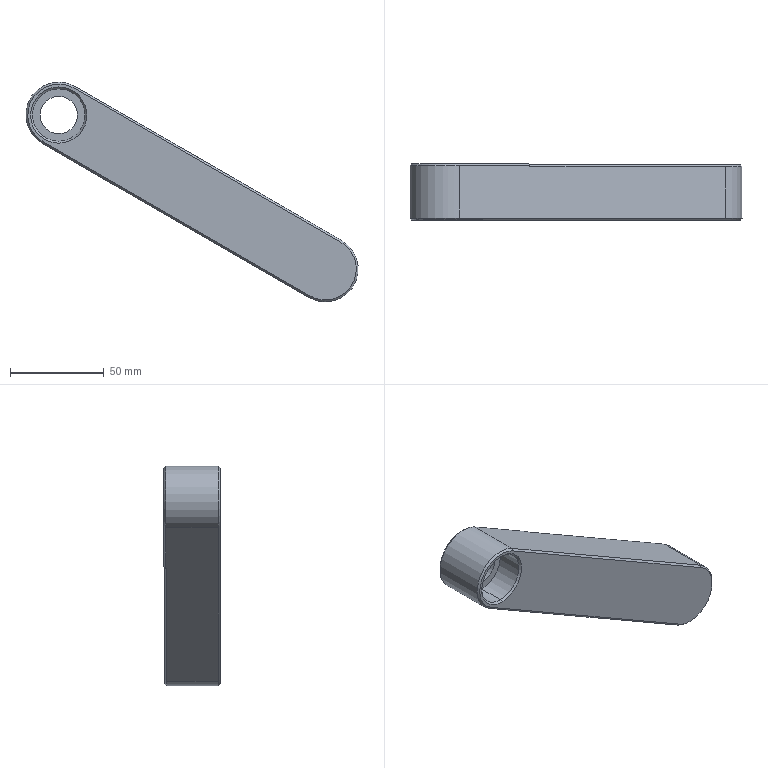Part | Creo | 1 solid | 27 faces | box 177.028 x 30 x 117 mm | volume 184252 mm3 | plane 13 | cone 8 | cylinder 6 | commonest cylinder face diameters 20 x2 28 x2 35 x2
STEP:
#1=CARTESIAN_POINT('',(0.,0.,0.));
#2=DIRECTION('',(0.,0.,1.));
#3=DIRECTION('',(1.,0.,0.));
#4=AXIS2_PLACEMENT_3D('',#1,#2,#3);
#5=CARTESIAN_POINT('',(85.75,-249.,-168.711));
#6=VERTEX_POINT('',#5);
#7=CARTESIAN_POINT('',(-56.278,-249.,-86.711));
#8=VERTEX_POINT('',#7);
#9=CARTESIAN_POINT('',(85.75,-249.,-168.711));
#10=DIRECTION('',(-0.866,0.,0.5));
#11=VECTOR('',#10,164.);
#12=LINE('',#9,#11);
#13=EDGE_CURVE('',#6,#8,#12,.T.);
#14=ORIENTED_EDGE('',*,*,#13,.F.);
#15=CARTESIAN_POINT('',(77.5,-249.,-199.5));
#16=VERTEX_POINT('',#15);
#17=CARTESIAN_POINT('',(77.5,-249.,-183.));
#18=DIRECTION('',(0.,-1.,0.));
#19=DIRECTION('',(0.,0.,-1.));
#20=AXIS2_PLACEMENT_3D('',#17,#18,#19);
#21=CIRCLE('',#20,16.5);
#22=EDGE_CURVE('',#16,#6,#21,.T.);
#23=ORIENTED_EDGE('',*,*,#22,.F.);
#24=CARTESIAN_POINT('',(69.25,-249.,-197.289));
#25=VERTEX_POINT('',#24);
#26=CARTESIAN_POINT('',(77.5,-249.,-183.));
#27=DIRECTION('',(0.,-1.,0.));
#28=DIRECTION('',(-0.5,0.,-0.866));
#29=AXIS2_PLACEMENT_3D('',#26,#27,#28);
#30=CIRCLE('',#29,16.5);
#31=EDGE_CURVE('',#25,#16,#30,.T.);
#32=ORIENTED_EDGE('',*,*,#31,.F.);
#33=CARTESIAN_POINT('',(-72.778,-249.,-115.289));
#34=VERTEX_POINT('',#33);
#35=CARTESIAN_POINT('',(-72.778,-249.,-115.289));
#36=DIRECTION('',(0.866,0.,-0.5));
#37=VECTOR('',#36,164.);
#38=LINE('',#35,#37);
#39=EDGE_CURVE('',#34,#25,#38,.T.);
#40=ORIENTED_EDGE('',*,*,#39,.F.);
#41=CARTESIAN_POINT('',(-64.528,-249.,-101.));
#42=DIRECTION('',(0.,-1.,0.));
#43=DIRECTION('',(0.5,0.,0.866));
#44=AXIS2_PLACEMENT_3D('',#41,#42,#43);
#45=CIRCLE('',#44,16.5);
#46=EDGE_CURVE('',#8,#34,#45,.T.);
#47=ORIENTED_EDGE('',*,*,#46,.F.);
#48=EDGE_LOOP('',(#14,#23,#32,#40,#47));
#49=FACE_OUTER_BOUND('',#48,.F.);
#50=CARTESIAN_POINT('',(-64.528,-249.,-86.));
#51=VERTEX_POINT('',#50);
#52=CARTESIAN_POINT('',(-64.528,-249.,-116.));
#53=VERTEX_POINT('',#52);
#54=CARTESIAN_POINT('',(-64.528,-249.,-101.));
#55=DIRECTION('',(0.,1.,0.));
#56=DIRECTION('',(0.,0.,1.));
#57=AXIS2_PLACEMENT_3D('',#54,#55,#56);
#58=CIRCLE('',#57,15.);
#59=EDGE_CURVE('',#51,#53,#58,.T.);
#60=ORIENTED_EDGE('',*,*,#59,.F.);
#61=CARTESIAN_POINT('',(-64.528,-249.,-101.));
#62=DIRECTION('',(0.,1.,0.));
#63=DIRECTION('',(0.,0.,-1.));
#64=AXIS2_PLACEMENT_3D('',#61,#62,#63);
#65=CIRCLE('',#64,15.);
#66=EDGE_CURVE('',#53,#51,#65,.T.);
#67=ORIENTED_EDGE('',*,*,#66,.F.);
#68=EDGE_LOOP('',(#60,#67));
#69=FACE_BOUND('',#68,.F.);
#70=CARTESIAN_POINT('',(-103.499,-249.,-78.5));
#71=DIRECTION('',(0.,-1.,0.));
#72=DIRECTION('',(0.,0.,-1.));
#73=AXIS2_PLACEMENT_3D('',#70,#71,#72);
#74=PLANE('',#73);
#75=ADVANCED_FACE('',(#49,#69),#74,.T.);
#76=CARTESIAN_POINT('',(-64.528,-248.,-87.));
#77=VERTEX_POINT('',#76);
#78=CARTESIAN_POINT('',(-64.528,-248.,-115.));
#79=VERTEX_POINT('',#78);
#80=CARTESIAN_POINT('',(-64.528,-248.,-101.));
#81=DIRECTION('',(0.,1.,0.));
#82=DIRECTION('',(0.,0.,1.));
#83=AXIS2_PLACEMENT_3D('',#80,#81,#82);
#84=CIRCLE('',#83,14.);
#85=EDGE_CURVE('',#77,#79,#84,.T.);
#86=ORIENTED_EDGE('',*,*,#85,.F.);
#87=CARTESIAN_POINT('',(-64.528,-248.,-87.));
#88=DIRECTION('',(0.,-0.7071,0.7071));
#89=VECTOR('',#88,1.414);
#90=LINE('',#87,#89);
#91=EDGE_CURVE('',#77,#51,#90,.T.);
#92=ORIENTED_EDGE('',*,*,#91,.T.);
#93=ORIENTED_EDGE('',*,*,#59,.T.);
#94=CARTESIAN_POINT('',(-64.528,-248.,-115.));
#95=DIRECTION('',(0.,-0.7071,-0.7071));
#96=VECTOR('',#95,1.414);
#97=LINE('',#94,#96);
#98=EDGE_CURVE('',#79,#53,#97,.T.);
#99=ORIENTED_EDGE('',*,*,#98,.F.);
#100=EDGE_LOOP('',(#86,#92,#93,#99));
#101=FACE_OUTER_BOUND('',#100,.F.);
#102=CARTESIAN_POINT('',(-64.528,-248.5,-101.));
#103=DIRECTION('',(0.,-1.,0.));
#104=DIRECTION('',(0.,0.,1.));
#105=AXIS2_PLACEMENT_3D('',#102,#103,#104);
#106=CONICAL_SURFACE('',#105,14.5,45.);
#107=ADVANCED_FACE('',(#101),#106,.F.);
#108=ORIENTED_EDGE('',*,*,#85,.T.);
#109=CARTESIAN_POINT('',(-64.528,-234.,-115.));
#110=VERTEX_POINT('',#109);
#111=CARTESIAN_POINT('',(-64.528,-248.,-115.));
#112=DIRECTION('',(0.,1.,0.));
#113=VECTOR('',#112,14.);
#114=LINE('',#111,#113);
#115=EDGE_CURVE('',#79,#110,#114,.T.);
#116=ORIENTED_EDGE('',*,*,#115,.T.);
#117=CARTESIAN_POINT('',(-64.528,-234.,-87.));
#118=VERTEX_POINT('',#117);
#119=CARTESIAN_POINT('',(-64.528,-234.,-101.));
#120=DIRECTION('',(0.,-1.,0.));
#121=DIRECTION('',(0.,0.,-1.));
#122=AXIS2_PLACEMENT_3D('',#119,#120,#121);
#123=CIRCLE('',#122,14.);
#124=EDGE_CURVE('',#110,#118,#123,.T.);
#125=ORIENTED_EDGE('',*,*,#124,.T.);
#126=CARTESIAN_POINT('',(-64.528,-248.,-87.));
#127=DIRECTION('',(0.,1.,0.));
#128=VECTOR('',#127,14.);
#129=LINE('',#126,#128);
#130=EDGE_CURVE('',#77,#118,#129,.T.);
#131=ORIENTED_EDGE('',*,*,#130,.F.);
#132=EDGE_LOOP('',(#108,#116,#125,#131));
#133=FACE_OUTER_BOUND('',#132,.F.);
#134=CARTESIAN_POINT('',(-64.528,-249.,-101.));
#135=DIRECTION('',(0.,1.,0.));
#136=DIRECTION('',(0.,0.,1.));
#137=AXIS2_PLACEMENT_3D('',#134,#135,#136);
#138=CYLINDRICAL_SURFACE('',#137,14.);
#139=ADVANCED_FACE('',(#133),#138,.F.);
#140=CARTESIAN_POINT('',(-64.528,-248.,-101.));
#141=DIRECTION('',(0.,1.,0.));
#142=DIRECTION('',(0.,0.,-1.));
#143=AXIS2_PLACEMENT_3D('',#140,#141,#142);
#144=CIRCLE('',#143,14.);
#145=EDGE_CURVE('',#79,#77,#144,.T.);
#146=ORIENTED_EDGE('',*,*,#145,.T.);
#147=ORIENTED_EDGE('',*,*,#130,.T.);
#148=CARTESIAN_POINT('',(-64.528,-234.,-101.));
#149=DIRECTION('',(0.,-1.,0.));
#150=DIRECTION('',(0.,0.,1.));
#151=AXIS2_PLACEMENT_3D('',#148,#149,#150);
#152=CIRCLE('',#151,14.);
#153=EDGE_CURVE('',#118,#110,#152,.T.);
#154=ORIENTED_EDGE('',*,*,#153,.T.);
#155=ORIENTED_EDGE('',*,*,#115,.F.);
#156=EDGE_LOOP('',(#146,#147,#154,#155));
#157=FACE_OUTER_BOUND('',#156,.F.);
#158=CARTESIAN_POINT('',(-64.528,-249.,-101.));
#159=DIRECTION('',(0.,1.,0.));
#160=DIRECTION('',(0.,0.,1.));
#161=AXIS2_PLACEMENT_3D('',#158,#159,#160);
#162=CYLINDRICAL_SURFACE('',#161,14.);
#163=ADVANCED_FACE('',(#157),#162,.F.);
#164=ORIENTED_EDGE('',*,*,#145,.F.);
#165=ORIENTED_EDGE('',*,*,#98,.T.);
#166=ORIENTED_EDGE('',*,*,#66,.T.);
#167=ORIENTED_EDGE('',*,*,#91,.F.);
#168=EDGE_LOOP('',(#164,#165,#166,#167));
#169=FACE_OUTER_BOUND('',#168,.F.);
#170=CARTESIAN_POINT('',(-64.528,-248.5,-101.));
#171=DIRECTION('',(0.,-1.,0.));
#172=DIRECTION('',(0.,0.,1.));
#173=AXIS2_PLACEMENT_3D('',#170,#171,#172);
#174=CONICAL_SURFACE('',#173,14.5,45.);
#175=ADVANCED_FACE('',(#169),#174,.F.);
#176=ORIENTED_EDGE('',*,*,#153,.F.);
#177=ORIENTED_EDGE('',*,*,#124,.F.);
#178=EDGE_LOOP('',(#176,#177));
#179=FACE_OUTER_BOUND('',#178,.F.);
#180=CARTESIAN_POINT('',(-64.528,-234.,-111.));
#181=VERTEX_POINT('',#180);
#182=CARTESIAN_POINT('',(-64.528,-234.,-91.));
#183=VERTEX_POINT('',#182);
#184=CARTESIAN_POINT('',(-64.528,-234.,-101.));
#185=DIRECTION('',(0.,1.,0.));
#186=DIRECTION('',(0.,0.,-1.));
#187=AXIS2_PLACEMENT_3D('',#184,#185,#186);
#188=CIRCLE('',#187,10.);
#189=EDGE_CURVE('',#181,#183,#188,.T.);
#190=ORIENTED_EDGE('',*,*,#189,.F.);
#191=CARTESIAN_POINT('',(-64.528,-234.,-101.));
#192=DIRECTION('',(0.,1.,0.));
#193=DIRECTION('',(0.,0.,1.));
#194=AXIS2_PLACEMENT_3D('',#191,#192,#193);
#195=CIRCLE('',#194,10.);
#196=EDGE_CURVE('',#183,#181,#195,.T.);
#197=ORIENTED_EDGE('',*,*,#196,.F.);
#198=EDGE_LOOP('',(#190,#197));
#199=FACE_BOUND('',#198,.F.);
#200=CARTESIAN_POINT('',(-64.528,-234.,-101.));
#201=DIRECTION('',(0.,-1.,0.));
#202=DIRECTION('',(0.,0.,-1.));
#203=AXIS2_PLACEMENT_3D('',#200,#201,#202);
#204=PLANE('',#203);
#205=ADVANCED_FACE('',(#179,#199),#204,.T.);
#206=CARTESIAN_POINT('',(-64.528,-220.,-91.));
#207=VERTEX_POINT('',#206);
#208=CARTESIAN_POINT('',(-64.528,-220.,-111.));
#209=VERTEX_POINT('',#208);
#210=CARTESIAN_POINT('',(-64.528,-220.,-101.));
#211=DIRECTION('',(0.,-1.,0.));
#212=DIRECTION('',(0.,0.,1.));
#213=AXIS2_PLACEMENT_3D('',#210,#211,#212);
#214=CIRCLE('',#213,10.);
#215=EDGE_CURVE('',#207,#209,#214,.T.);
#216=ORIENTED_EDGE('',*,*,#215,.T.);
#217=CARTESIAN_POINT('',(-64.528,-234.,-111.));
#218=DIRECTION('',(0.,1.,0.));
#219=VECTOR('',#218,14.);
#220=LINE('',#217,#219);
#221=EDGE_CURVE('',#181,#209,#220,.T.);
#222=ORIENTED_EDGE('',*,*,#221,.F.);
#223=ORIENTED_EDGE('',*,*,#189,.T.);
#224=CARTESIAN_POINT('',(-64.528,-234.,-91.));
#225=DIRECTION('',(0.,1.,0.));
#226=VECTOR('',#225,14.);
#227=LINE('',#224,#226);
#228=EDGE_CURVE('',#183,#207,#227,.T.);
#229=ORIENTED_EDGE('',*,*,#228,.T.);
#230=EDGE_LOOP('',(#216,#222,#223,#229));
#231=FACE_OUTER_BOUND('',#230,.F.);
#232=CARTESIAN_POINT('',(-64.528,-249.,-101.));
#233=DIRECTION('',(0.,1.,0.));
#234=DIRECTION('',(0.,0.,1.));
#235=AXIS2_PLACEMENT_3D('',#232,#233,#234);
#236=CYLINDRICAL_SURFACE('',#235,10.);
#237=ADVANCED_FACE('',(#231),#236,.F.);
#238=CARTESIAN_POINT('',(-64.528,-219.,-90.));
#239=VERTEX_POINT('',#238);
#240=CARTESIAN_POINT('',(-64.528,-219.,-112.));
#241=VERTEX_POINT('',#240);
#242=CARTESIAN_POINT('',(-64.528,-219.,-101.));
#243=DIRECTION('',(0.,-1.,0.));
#244=DIRECTION('',(0.,0.,1.));
#245=AXIS2_PLACEMENT_3D('',#242,#243,#244);
#246=CIRCLE('',#245,11.);
#247=EDGE_CURVE('',#239,#241,#246,.T.);
#248=ORIENTED_EDGE('',*,*,#247,.T.);
#249=CARTESIAN_POINT('',(-64.528,-220.,-111.));
#250=DIRECTION('',(0.,0.7071,-0.7071));
#251=VECTOR('',#250,1.414);
#252=LINE('',#249,#251);
#253=EDGE_CURVE('',#209,#241,#252,.T.);
#254=ORIENTED_EDGE('',*,*,#253,.F.);
#255=ORIENTED_EDGE('',*,*,#215,.F.);
#256=CARTESIAN_POINT('',(-64.528,-220.,-91.));
#257=DIRECTION('',(0.,0.7071,0.7071));
#258=VECTOR('',#257,1.414);
#259=LINE('',#256,#258);
#260=EDGE_CURVE('',#207,#239,#259,.T.);
#261=ORIENTED_EDGE('',*,*,#260,.T.);
#262=EDGE_LOOP('',(#248,#254,#255,#261));
#263=FACE_OUTER_BOUND('',#262,.F.);
#264=CARTESIAN_POINT('',(-64.528,-219.5,-101.));
#265=DIRECTION('',(0.,1.,0.));
#266=DIRECTION('',(0.,0.,-1.));
#267=AXIS2_PLACEMENT_3D('',#264,#265,#266);
#268=CONICAL_SURFACE('',#267,10.5,45.);
#269=ADVANCED_FACE('',(#263),#268,.F.);
#270=CARTESIAN_POINT('',(-72.778,-219.,-115.289));
#271=VERTEX_POINT('',#270);
#272=CARTESIAN_POINT('',(-56.278,-219.,-86.711));
#273=VERTEX_POINT('',#272);
#274=CARTESIAN_POINT('',(-64.528,-219.,-101.));
#275=DIRECTION('',(0.,1.,0.));
#276=DIRECTION('',(-0.5,0.,-0.866));
#277=AXIS2_PLACEMENT_3D('',#274,#275,#276);
#278=CIRCLE('',#277,16.5);
#279=EDGE_CURVE('',#271,#273,#278,.T.);
#280=ORIENTED_EDGE('',*,*,#279,.F.);
#281=CARTESIAN_POINT('',(-35.106,-219.,-137.039));
#282=VERTEX_POINT('',#281);
#283=CARTESIAN_POINT('',(-35.106,-219.,-137.039));
#284=DIRECTION('',(-0.866,0.,0.5));
#285=VECTOR('',#284,43.5);
#286=LINE('',#283,#285);
#287=EDGE_CURVE('',#282,#271,#286,.T.);
#288=ORIENTED_EDGE('',*,*,#287,.F.);
#289=CARTESIAN_POINT('',(-18.606,-219.,-108.461));
#290=VERTEX_POINT('',#289);
#291=CARTESIAN_POINT('',(-18.606,-219.,-108.461));
#292=DIRECTION('',(-0.5,0.,-0.866));
#293=VECTOR('',#292,33.);
#294=LINE('',#291,#293);
#295=EDGE_CURVE('',#290,#282,#294,.T.);
#296=ORIENTED_EDGE('',*,*,#295,.F.);
#297=CARTESIAN_POINT('',(-56.278,-219.,-86.711));
#298=DIRECTION('',(0.866,0.,-0.5));
#299=VECTOR('',#298,43.5);
#300=LINE('',#297,#299);
#301=EDGE_CURVE('',#273,#290,#300,.T.);
#302=ORIENTED_EDGE('',*,*,#301,.F.);
#303=EDGE_LOOP('',(#280,#288,#296,#302));
#304=FACE_OUTER_BOUND('',#303,.F.);
#305=ORIENTED_EDGE('',*,*,#247,.F.);
#306=CARTESIAN_POINT('',(-64.528,-219.,-101.));
#307=DIRECTION('',(0.,-1.,0.));
#308=DIRECTION('',(0.,0.,-1.));
#309=AXIS2_PLACEMENT_3D('',#306,#307,#308);
#310=CIRCLE('',#309,11.);
#311=EDGE_CURVE('',#241,#239,#310,.T.);
#312=ORIENTED_EDGE('',*,*,#311,.F.);
#313=EDGE_LOOP('',(#305,#312));
#314=FACE_BOUND('',#313,.F.);
#315=CARTESIAN_POINT('',(-94.839,-219.,-83.5));
#316=DIRECTION('',(0.,-1.,0.));
#317=DIRECTION('',(0.,0.,-1.));
#318=AXIS2_PLACEMENT_3D('',#315,#316,#317);
#319=PLANE('',#318);
#320=ADVANCED_FACE('',(#304,#314),#319,.F.);
#321=ORIENTED_EDGE('',*,*,#311,.T.);
#322=ORIENTED_EDGE('',*,*,#260,.F.);
#323=CARTESIAN_POINT('',(-64.528,-220.,-101.));
#324=DIRECTION('',(0.,-1.,0.));
#325=DIRECTION('',(0.,0.,-1.));
#326=AXIS2_PLACEMENT_3D('',#323,#324,#325);
#327=CIRCLE('',#326,10.);
#328=EDGE_CURVE('',#209,#207,#327,.T.);
#329=ORIENTED_EDGE('',*,*,#328,.F.);
#330=ORIENTED_EDGE('',*,*,#253,.T.);
#331=EDGE_LOOP('',(#321,#322,#329,#330));
#332=FACE_OUTER_BOUND('',#331,.F.);
#333=CARTESIAN_POINT('',(-64.528,-219.5,-101.));
#334=DIRECTION('',(0.,1.,0.));
#335=DIRECTION('',(0.,0.,-1.));
#336=AXIS2_PLACEMENT_3D('',#333,#334,#335);
#337=CONICAL_SURFACE('',#336,10.5,45.);
#338=ADVANCED_FACE('',(#332),#337,.F.);
#339=ORIENTED_EDGE('',*,*,#328,.T.);
#340=ORIENTED_EDGE('',*,*,#228,.F.);
#341=ORIENTED_EDGE('',*,*,#196,.T.);
#342=ORIENTED_EDGE('',*,*,#221,.T.);
#343=EDGE_LOOP('',(#339,#340,#341,#342));
#344=FACE_OUTER_BOUND('',#343,.F.);
#345=CARTESIAN_POINT('',(-64.528,-249.,-101.));
#346=DIRECTION('',(0.,1.,0.));
#347=DIRECTION('',(0.,0.,1.));
#348=AXIS2_PLACEMENT_3D('',#345,#346,#347);
#349=CYLINDRICAL_SURFACE('',#348,10.);
#350=ADVANCED_FACE('',(#344),#349,.F.);
#351=CARTESIAN_POINT('',(-73.278,-220.,-116.155));
#352=VERTEX_POINT('',#351);
#353=CARTESIAN_POINT('',(-72.778,-219.,-115.289));
#354=DIRECTION('',(-0.3536,-0.7071,-0.6124));
#355=VECTOR('',#354,1.414);
#356=LINE('',#353,#355);
#357=EDGE_CURVE('',#271,#352,#356,.T.);
#358=ORIENTED_EDGE('',*,*,#357,.F.);
#359=ORIENTED_EDGE('',*,*,#279,.T.);
#360=CARTESIAN_POINT('',(-55.778,-220.,-85.845));
#361=VERTEX_POINT('',#360);
#362=CARTESIAN_POINT('',(-55.778,-220.,-85.845));
#363=DIRECTION('',(-0.3536,0.7071,-0.6124));
#364=VECTOR('',#363,1.414);
#365=LINE('',#362,#364);
#366=EDGE_CURVE('',#361,#273,#365,.T.);
#367=ORIENTED_EDGE('',*,*,#366,.F.);
#368=CARTESIAN_POINT('',(-64.528,-220.,-83.5));
#369=VERTEX_POINT('',#368);
#370=CARTESIAN_POINT('',(-64.528,-220.,-101.));
#371=DIRECTION('',(0.,1.,0.));
#372=DIRECTION('',(0.,0.,1.));
#373=AXIS2_PLACEMENT_3D('',#370,#371,#372);
#374=CIRCLE('',#373,17.5);
#375=EDGE_CURVE('',#369,#361,#374,.T.);
#376=ORIENTED_EDGE('',*,*,#375,.F.);
#377=CARTESIAN_POINT('',(-64.528,-220.,-101.));
#378=DIRECTION('',(0.,1.,0.));
#379=DIRECTION('',(-0.5,0.,-0.866));
#380=AXIS2_PLACEMENT_3D('',#377,#378,#379);
#381=CIRCLE('',#380,17.5);
#382=EDGE_CURVE('',#352,#369,#381,.T.);
#383=ORIENTED_EDGE('',*,*,#382,.F.);
#384=EDGE_LOOP('',(#358,#359,#367,#376,#383));
#385=FACE_OUTER_BOUND('',#384,.F.);
#386=CARTESIAN_POINT('',(-64.528,-219.5,-101.));
#387=DIRECTION('',(0.,-1.,0.));
#388=DIRECTION('',(0.,0.,1.));
#389=AXIS2_PLACEMENT_3D('',#386,#387,#388);
#390=CONICAL_SURFACE('',#389,17.,45.);
#391=ADVANCED_FACE('',(#385),#390,.T.);
#392=ORIENTED_EDGE('',*,*,#287,.T.);
#393=ORIENTED_EDGE('',*,*,#357,.T.);
#394=CARTESIAN_POINT('',(-35.606,-220.,-137.905));
#395=VERTEX_POINT('',#394);
#396=CARTESIAN_POINT('',(-35.606,-220.,-137.905));
#397=DIRECTION('',(-0.866,0.,0.5));
#398=VECTOR('',#397,43.5);
#399=LINE('',#396,#398);
#400=EDGE_CURVE('',#395,#352,#399,.T.);
#401=ORIENTED_EDGE('',*,*,#400,.F.);
#402=CARTESIAN_POINT('',(-35.606,-220.,-137.905));
#403=DIRECTION('',(0.3536,0.7071,0.6124));
#404=VECTOR('',#403,1.414);
#405=LINE('',#402,#404);
#406=EDGE_CURVE('',#395,#282,#405,.T.);
#407=ORIENTED_EDGE('',*,*,#406,.T.);
#408=EDGE_LOOP('',(#392,#393,#401,#407));
#409=FACE_OUTER_BOUND('',#408,.F.);
#410=CARTESIAN_POINT('',(-103.589,-220.,-98.655));
#411=DIRECTION('',(-0.3536,0.7071,-0.6124));
#412=DIRECTION('',(-0.866,0.,0.5));
#413=AXIS2_PLACEMENT_3D('',#410,#411,#412);
#414=PLANE('',#413);
#415=ADVANCED_FACE('',(#409),#414,.T.);
#416=CARTESIAN_POINT('',(-73.278,-248.,-116.155));
#417=VERTEX_POINT('',#416);
#418=CARTESIAN_POINT('',(68.75,-248.,-198.155));
#419=VERTEX_POINT('',#418);
#420=CARTESIAN_POINT('',(-73.278,-248.,-116.155));
#421=DIRECTION('',(0.866,0.,-0.5));
#422=VECTOR('',#421,164.);
#423=LINE('',#420,#422);
#424=EDGE_CURVE('',#417,#419,#423,.T.);
#425=ORIENTED_EDGE('',*,*,#424,.T.);
#426=CARTESIAN_POINT('',(68.75,-220.5,-198.155));
#427=VERTEX_POINT('',#426);
#428=CARTESIAN_POINT('',(68.75,-248.,-198.155));
#429=DIRECTION('',(0.,1.,0.));
#430=VECTOR('',#429,27.5);
#431=LINE('',#428,#430);
#432=EDGE_CURVE('',#419,#427,#431,.T.);
#433=ORIENTED_EDGE('',*,*,#432,.T.);
#434=CARTESIAN_POINT('',(-35.606,-220.5,-137.905));
#435=VERTEX_POINT('',#434);
#436=CARTESIAN_POINT('',(68.75,-220.5,-198.155));
#437=DIRECTION('',(-0.866,0.,0.5));
#438=VECTOR('',#437,120.5);
#439=LINE('',#436,#438);
#440=EDGE_CURVE('',#427,#435,#439,.T.);
#441=ORIENTED_EDGE('',*,*,#440,.T.);
#442=CARTESIAN_POINT('',(-35.606,-220.,-137.905));
#443=DIRECTION('',(0.,-1.,0.));
#444=VECTOR('',#443,0.5);
#445=LINE('',#442,#444);
#446=EDGE_CURVE('',#395,#435,#445,.T.);
#447=ORIENTED_EDGE('',*,*,#446,.F.);
#448=ORIENTED_EDGE('',*,*,#400,.T.);
#449=CARTESIAN_POINT('',(-73.278,-220.,-116.155));
#450=DIRECTION('',(0.,-1.,0.));
#451=VECTOR('',#450,28.);
#452=LINE('',#449,#451);
#453=EDGE_CURVE('',#352,#417,#452,.T.);
#454=ORIENTED_EDGE('',*,*,#453,.T.);
#455=EDGE_LOOP('',(#425,#433,#441,#447,#448,#454));
#456=FACE_OUTER_BOUND('',#455,.F.);
#457=CARTESIAN_POINT('',(-112.249,-219.,-93.655));
#458=DIRECTION('',(-0.5,0.,-0.866));
#459=DIRECTION('',(-0.866,0.,0.5));
#460=AXIS2_PLACEMENT_3D('',#457,#458,#459);
#461=PLANE('',#460);
#462=ADVANCED_FACE('',(#456),#461,.T.);
#463=ORIENTED_EDGE('',*,*,#39,.T.);
#464=CARTESIAN_POINT('',(69.25,-249.,-197.289));
#465=DIRECTION('',(-0.3536,0.7071,-0.6124));
#466=VECTOR('',#465,1.414);
#467=LINE('',#464,#466);
#468=EDGE_CURVE('',#25,#419,#467,.T.);
#469=ORIENTED_EDGE('',*,*,#468,.T.);
#470=ORIENTED_EDGE('',*,*,#424,.F.);
#471=CARTESIAN_POINT('',(-73.278,-248.,-116.155));
#472=DIRECTION('',(0.3536,-0.7071,0.6124));
#473=VECTOR('',#472,1.414);
#474=LINE('',#471,#473);
#475=EDGE_CURVE('',#417,#34,#474,.T.);
#476=ORIENTED_EDGE('',*,*,#475,.T.);
#477=EDGE_LOOP('',(#463,#469,#470,#476));
#478=FACE_OUTER_BOUND('',#477,.F.);
#479=CARTESIAN_POINT('',(-112.249,-248.,-93.655));
#480=DIRECTION('',(0.3536,0.7071,0.6124));
#481=DIRECTION('',(-0.866,0.,0.5));
#482=AXIS2_PLACEMENT_3D('',#479,#480,#481);
#483=PLANE('',#482);
#484=ADVANCED_FACE('',(#478),#483,.F.);
#485=CARTESIAN_POINT('',(86.25,-248.,-167.845));
#486=VERTEX_POINT('',#485);
#487=CARTESIAN_POINT('',(86.25,-248.,-167.845));
#488=DIRECTION('',(-0.3536,-0.7071,-0.6124));
#489=VECTOR('',#488,1.414);
#490=LINE('',#487,#489);
#491=EDGE_CURVE('',#486,#6,#490,.T.);
#492=ORIENTED_EDGE('',*,*,#491,.F.);
#493=CARTESIAN_POINT('',(77.5,-248.,-200.5));
#494=VERTEX_POINT('',#493);
#495=CARTESIAN_POINT('',(77.5,-248.,-183.));
#496=DIRECTION('',(0.,-1.,0.));
#497=DIRECTION('',(0.,0.,-1.));
#498=AXIS2_PLACEMENT_3D('',#495,#496,#497);
#499=CIRCLE('',#498,17.5);
#500=EDGE_CURVE('',#494,#486,#499,.T.);
#501=ORIENTED_EDGE('',*,*,#500,.F.);
#502=CARTESIAN_POINT('',(77.5,-248.,-183.));
#503=DIRECTION('',(0.,-1.,0.));
#504=DIRECTION('',(-0.5,0.,-0.866));
#505=AXIS2_PLACEMENT_3D('',#502,#503,#504);
#506=CIRCLE('',#505,17.5);
#507=EDGE_CURVE('',#419,#494,#506,.T.);
#508=ORIENTED_EDGE('',*,*,#507,.F.);
#509=ORIENTED_EDGE('',*,*,#468,.F.);
#510=ORIENTED_EDGE('',*,*,#31,.T.);
#511=ORIENTED_EDGE('',*,*,#22,.T.);
#512=EDGE_LOOP('',(#492,#501,#508,#509,#510,#511));
#513=FACE_OUTER_BOUND('',#512,.F.);
#514=CARTESIAN_POINT('',(77.5,-248.5,-183.));
#515=DIRECTION('',(0.,1.,0.));
#516=DIRECTION('',(0.,0.,-1.));
#517=AXIS2_PLACEMENT_3D('',#514,#515,#516);
#518=CONICAL_SURFACE('',#517,17.,45.);
#519=ADVANCED_FACE('',(#513),#518,.T.);
#520=CARTESIAN_POINT('',(-55.778,-248.,-85.845));
#521=VERTEX_POINT('',#520);
#522=CARTESIAN_POINT('',(86.25,-248.,-167.845));
#523=DIRECTION('',(-0.866,0.,0.5));
#524=VECTOR('',#523,164.);
#525=LINE('',#522,#524);
#526=EDGE_CURVE('',#486,#521,#525,.T.);
#527=ORIENTED_EDGE('',*,*,#526,.F.);
#528=ORIENTED_EDGE('',*,*,#491,.T.);
#529=ORIENTED_EDGE('',*,*,#13,.T.);
#530=CARTESIAN_POINT('',(-56.278,-249.,-86.711));
#531=DIRECTION('',(0.3536,0.7071,0.6124));
#532=VECTOR('',#531,1.414);
#533=LINE('',#530,#532);
#534=EDGE_CURVE('',#8,#521,#533,.T.);
#535=ORIENTED_EDGE('',*,*,#534,.T.);
#536=EDGE_LOOP('',(#527,#528,#529,#535));
#537=FACE_OUTER_BOUND('',#536,.F.);
#538=CARTESIAN_POINT('',(-94.749,-248.,-63.345));
#539=DIRECTION('',(0.3536,-0.7071,0.6124));
#540=DIRECTION('',(-0.866,0.,0.5));
#541=AXIS2_PLACEMENT_3D('',#538,#539,#540);
#542=PLANE('',#541);
#543=ADVANCED_FACE('',(#537),#542,.T.);
#544=CARTESIAN_POINT('',(86.25,-220.5,-167.845));
#545=VERTEX_POINT('',#544);
#546=CARTESIAN_POINT('',(86.25,-220.5,-167.845));
#547=DIRECTION('',(0.,-1.,0.));
#548=VECTOR('',#547,27.5);
#549=LINE('',#546,#548);
#550=EDGE_CURVE('',#545,#486,#549,.T.);
#551=ORIENTED_EDGE('',*,*,#550,.T.);
#552=ORIENTED_EDGE('',*,*,#526,.T.);
#553=CARTESIAN_POINT('',(-55.778,-248.,-85.845));
#554=DIRECTION('',(0.,1.,0.));
#555=VECTOR('',#554,28.);
#556=LINE('',#553,#555);
#557=EDGE_CURVE('',#521,#361,#556,.T.);
#558=ORIENTED_EDGE('',*,*,#557,.T.);
#559=CARTESIAN_POINT('',(-18.106,-220.,-107.595));
#560=VERTEX_POINT('',#559);
#561=CARTESIAN_POINT('',(-55.778,-220.,-85.845));
#562=DIRECTION('',(0.866,0.,-0.5));
#563=VECTOR('',#562,43.5);
#564=LINE('',#561,#563);
#565=EDGE_CURVE('',#361,#560,#564,.T.);
#566=ORIENTED_EDGE('',*,*,#565,.T.);
#567=CARTESIAN_POINT('',(-18.106,-220.5,-107.595));
#568=VERTEX_POINT('',#567);
#569=CARTESIAN_POINT('',(-18.106,-220.5,-107.595));
#570=DIRECTION('',(0.,1.,0.));
#571=VECTOR('',#570,0.5);
#572=LINE('',#569,#571);
#573=EDGE_CURVE('',#568,#560,#572,.T.);
#574=ORIENTED_EDGE('',*,*,#573,.F.);
#575=CARTESIAN_POINT('',(-18.106,-220.5,-107.595));
#576=DIRECTION('',(0.866,0.,-0.5));
#577=VECTOR('',#576,120.5);
#578=LINE('',#575,#577);
#579=EDGE_CURVE('',#568,#545,#578,.T.);
#580=ORIENTED_EDGE('',*,*,#579,.T.);
#581=EDGE_LOOP('',(#551,#552,#558,#566,#574,#580));
#582=FACE_OUTER_BOUND('',#581,.F.);
#583=CARTESIAN_POINT('',(-94.749,-219.,-63.345));
#584=DIRECTION('',(-0.5,0.,-0.866));
#585=DIRECTION('',(-0.866,0.,0.5));
#586=AXIS2_PLACEMENT_3D('',#583,#584,#585);
#587=PLANE('',#586);
#588=ADVANCED_FACE('',(#582),#587,.F.);
#589=ORIENTED_EDGE('',*,*,#432,.F.);
#590=ORIENTED_EDGE('',*,*,#507,.T.);
#591=ORIENTED_EDGE('',*,*,#500,.T.);
#592=ORIENTED_EDGE('',*,*,#550,.F.);
#593=CARTESIAN_POINT('',(77.5,-220.5,-200.5));
#594=VERTEX_POINT('',#593);
#595=CARTESIAN_POINT('',(77.5,-220.5,-183.));
#596=DIRECTION('',(0.,1.,0.));
#597=DIRECTION('',(0.5,0.,0.866));
#598=AXIS2_PLACEMENT_3D('',#595,#596,#597);
#599=CIRCLE('',#598,17.5);
#600=EDGE_CURVE('',#545,#594,#599,.T.);
#601=ORIENTED_EDGE('',*,*,#600,.T.);
#602=CARTESIAN_POINT('',(77.5,-220.5,-183.));
#603=DIRECTION('',(0.,1.,0.));
#604=DIRECTION('',(0.,0.,-1.));
#605=AXIS2_PLACEMENT_3D('',#602,#603,#604);
#606=CIRCLE('',#605,17.5);
#607=EDGE_CURVE('',#594,#427,#606,.T.);
#608=ORIENTED_EDGE('',*,*,#607,.T.);
#609=EDGE_LOOP('',(#589,#590,#591,#592,#601,#608));
#610=FACE_OUTER_BOUND('',#609,.F.);
#611=CARTESIAN_POINT('',(77.5,-249.,-183.));
#612=DIRECTION('',(0.,1.,0.));
#613=DIRECTION('',(0.,0.,1.));
#614=AXIS2_PLACEMENT_3D('',#611,#612,#613);
#615=CYLINDRICAL_SURFACE('',#614,17.5);
#616=ADVANCED_FACE('',(#610),#615,.T.);
#617=CARTESIAN_POINT('',(69.25,-219.5,-197.289));
#618=VERTEX_POINT('',#617);
#619=CARTESIAN_POINT('',(68.75,-220.5,-198.155));
#620=DIRECTION('',(0.3536,0.7071,0.6124));
#621=VECTOR('',#620,1.414);
#622=LINE('',#619,#621);
#623=EDGE_CURVE('',#427,#618,#622,.T.);
#624=ORIENTED_EDGE('',*,*,#623,.F.);
#625=ORIENTED_EDGE('',*,*,#607,.F.);
#626=ORIENTED_EDGE('',*,*,#600,.F.);
#627=CARTESIAN_POINT('',(85.75,-219.5,-168.711));
#628=VERTEX_POINT('',#627);
#629=CARTESIAN_POINT('',(85.75,-219.5,-168.711));
#630=DIRECTION('',(0.3536,-0.7071,0.6124));
#631=VECTOR('',#630,1.414);
#632=LINE('',#629,#631);
#633=EDGE_CURVE('',#628,#545,#632,.T.);
#634=ORIENTED_EDGE('',*,*,#633,.F.);
#635=CARTESIAN_POINT('',(77.5,-219.5,-199.5));
#636=VERTEX_POINT('',#635);
#637=CARTESIAN_POINT('',(77.5,-219.5,-183.));
#638=DIRECTION('',(0.,1.,0.));
#639=DIRECTION('',(0.5,0.,0.866));
#640=AXIS2_PLACEMENT_3D('',#637,#638,#639);
#641=CIRCLE('',#640,16.5);
#642=EDGE_CURVE('',#628,#636,#641,.T.);
#643=ORIENTED_EDGE('',*,*,#642,.T.);
#644=CARTESIAN_POINT('',(77.5,-219.5,-183.));
#645=DIRECTION('',(0.,1.,0.));
#646=DIRECTION('',(0.,0.,-1.));
#647=AXIS2_PLACEMENT_3D('',#644,#645,#646);
#648=CIRCLE('',#647,16.5);
#649=EDGE_CURVE('',#636,#618,#648,.T.);
#650=ORIENTED_EDGE('',*,*,#649,.T.);
#651=EDGE_LOOP('',(#624,#625,#626,#634,#643,#650));
#652=FACE_OUTER_BOUND('',#651,.F.);
#653=CARTESIAN_POINT('',(77.5,-220.,-183.));
#654=DIRECTION('',(0.,-1.,0.));
#655=DIRECTION('',(0.,0.,1.));
#656=AXIS2_PLACEMENT_3D('',#653,#654,#655);
#657=CONICAL_SURFACE('',#656,17.,45.);
#658=ADVANCED_FACE('',(#652),#657,.T.);
#659=CARTESIAN_POINT('',(-35.106,-219.5,-137.039));
#660=VERTEX_POINT('',#659);
#661=CARTESIAN_POINT('',(-35.106,-219.5,-137.039));
#662=DIRECTION('',(-0.3536,-0.7071,-0.6124));
#663=VECTOR('',#662,1.414);
#664=LINE('',#661,#663);
#665=EDGE_CURVE('',#660,#435,#664,.T.);
#666=ORIENTED_EDGE('',*,*,#665,.T.);
#667=ORIENTED_EDGE('',*,*,#440,.F.);
#668=ORIENTED_EDGE('',*,*,#623,.T.);
#669=CARTESIAN_POINT('',(69.25,-219.5,-197.289));
#670=DIRECTION('',(-0.866,0.,0.5));
#671=VECTOR('',#670,120.5);
#672=LINE('',#669,#671);
#673=EDGE_CURVE('',#618,#660,#672,.T.);
#674=ORIENTED_EDGE('',*,*,#673,.T.);
#675=EDGE_LOOP('',(#666,#667,#668,#674));
#676=FACE_OUTER_BOUND('',#675,.F.);
#677=CARTESIAN_POINT('',(-112.249,-220.5,-93.655));
#678=DIRECTION('',(-0.3536,0.7071,-0.6124));
#679=DIRECTION('',(-0.866,0.,0.5));
#680=AXIS2_PLACEMENT_3D('',#677,#678,#679);
#681=PLANE('',#680);
#682=ADVANCED_FACE('',(#676),#681,.T.);
#683=ORIENTED_EDGE('',*,*,#573,.T.);
#684=CARTESIAN_POINT('',(-18.606,-219.,-108.461));
#685=DIRECTION('',(0.3536,-0.7071,0.6124));
#686=VECTOR('',#685,1.414);
#687=LINE('',#684,#686);
#688=EDGE_CURVE('',#290,#560,#687,.T.);
#689=ORIENTED_EDGE('',*,*,#688,.F.);
#690=ORIENTED_EDGE('',*,*,#295,.T.);
#691=ORIENTED_EDGE('',*,*,#406,.F.);
#692=ORIENTED_EDGE('',*,*,#446,.T.);
#693=ORIENTED_EDGE('',*,*,#665,.F.);
#694=CARTESIAN_POINT('',(-18.606,-219.5,-108.461));
#695=VERTEX_POINT('',#694);
#696=CARTESIAN_POINT('',(-35.106,-219.5,-137.039));
#697=DIRECTION('',(0.5,0.,0.866));
#698=VECTOR('',#697,33.);
#699=LINE('',#696,#698);
#700=EDGE_CURVE('',#660,#695,#699,.T.);
#701=ORIENTED_EDGE('',*,*,#700,.T.);
#702=CARTESIAN_POINT('',(-18.106,-220.5,-107.595));
#703=DIRECTION('',(-0.3536,0.7071,-0.6124));
#704=VECTOR('',#703,1.414);
#705=LINE('',#702,#704);
#706=EDGE_CURVE('',#568,#695,#705,.T.);
#707=ORIENTED_EDGE('',*,*,#706,.F.);
#708=EDGE_LOOP('',(#683,#689,#690,#691,#692,#693,#701,#707));
#709=FACE_OUTER_BOUND('',#708,.F.);
#710=CARTESIAN_POINT('',(-26.856,-218.,-122.75));
#711=DIRECTION('',(-0.866,0.,0.5));
#712=DIRECTION('',(-0.5,0.,-0.866));
#713=AXIS2_PLACEMENT_3D('',#710,#711,#712);
#714=PLANE('',#713);
#715=ADVANCED_FACE('',(#709),#714,.F.);
#716=ORIENTED_EDGE('',*,*,#565,.F.);
#717=ORIENTED_EDGE('',*,*,#366,.T.);
#718=ORIENTED_EDGE('',*,*,#301,.T.);
#719=ORIENTED_EDGE('',*,*,#688,.T.);
#720=EDGE_LOOP('',(#716,#717,#718,#719));
#721=FACE_OUTER_BOUND('',#720,.F.);
#722=CARTESIAN_POINT('',(-86.089,-220.,-68.345));
#723=DIRECTION('',(-0.3536,-0.7071,-0.6124));
#724=DIRECTION('',(-0.866,0.,0.5));
#725=AXIS2_PLACEMENT_3D('',#722,#723,#724);
#726=PLANE('',#725);
#727=ADVANCED_FACE('',(#721),#726,.F.);
#728=ORIENTED_EDGE('',*,*,#700,.F.);
#729=ORIENTED_EDGE('',*,*,#673,.F.);
#730=ORIENTED_EDGE('',*,*,#649,.F.);
#731=ORIENTED_EDGE('',*,*,#642,.F.);
#732=CARTESIAN_POINT('',(-18.606,-219.5,-108.461));
#733=DIRECTION('',(0.866,0.,-0.5));
#734=VECTOR('',#733,120.5);
#735=LINE('',#732,#734);
#736=EDGE_CURVE('',#695,#628,#735,.T.);
#737=ORIENTED_EDGE('',*,*,#736,.F.);
#738=EDGE_LOOP('',(#728,#729,#730,#731,#737));
#739=FACE_OUTER_BOUND('',#738,.F.);
#740=CARTESIAN_POINT('',(2.156,-219.5,-139.5));
#741=DIRECTION('',(0.,-1.,0.));
#742=DIRECTION('',(0.,0.,1.));
#743=AXIS2_PLACEMENT_3D('',#740,#741,#742);
#744=PLANE('',#743);
#745=ADVANCED_FACE('',(#739),#744,.F.);
#746=ORIENTED_EDGE('',*,*,#633,.T.);
#747=ORIENTED_EDGE('',*,*,#579,.F.);
#748=ORIENTED_EDGE('',*,*,#706,.T.);
#749=ORIENTED_EDGE('',*,*,#736,.T.);
#750=EDGE_LOOP('',(#746,#747,#748,#749));
#751=FACE_OUTER_BOUND('',#750,.F.);
#752=CARTESIAN_POINT('',(-94.749,-220.5,-63.345));
#753=DIRECTION('',(-0.3536,-0.7071,-0.6124));
#754=DIRECTION('',(-0.866,0.,0.5));
#755=AXIS2_PLACEMENT_3D('',#752,#753,#754);
#756=PLANE('',#755);
#757=ADVANCED_FACE('',(#751),#756,.F.);
#758=ORIENTED_EDGE('',*,*,#453,.F.);
#759=ORIENTED_EDGE('',*,*,#382,.T.);
#760=ORIENTED_EDGE('',*,*,#375,.T.);
#761=ORIENTED_EDGE('',*,*,#557,.F.);
#762=CARTESIAN_POINT('',(-64.528,-248.,-83.5));
#763=VERTEX_POINT('',#762);
#764=CARTESIAN_POINT('',(-64.528,-248.,-101.));
#765=DIRECTION('',(0.,-1.,0.));
#766=DIRECTION('',(0.5,0.,0.866));
#767=AXIS2_PLACEMENT_3D('',#764,#765,#766);
#768=CIRCLE('',#767,17.5);
#769=EDGE_CURVE('',#521,#763,#768,.T.);
#770=ORIENTED_EDGE('',*,*,#769,.T.);
#771=CARTESIAN_POINT('',(-64.528,-248.,-101.));
#772=DIRECTION('',(0.,-1.,0.));
#773=DIRECTION('',(0.,0.,1.));
#774=AXIS2_PLACEMENT_3D('',#771,#772,#773);
#775=CIRCLE('',#774,17.5);
#776=EDGE_CURVE('',#763,#417,#775,.T.);
#777=ORIENTED_EDGE('',*,*,#776,.T.);
#778=EDGE_LOOP('',(#758,#759,#760,#761,#770,#777));
#779=FACE_OUTER_BOUND('',#778,.F.);
#780=CARTESIAN_POINT('',(-64.528,-249.,-101.));
#781=DIRECTION('',(0.,1.,0.));
#782=DIRECTION('',(0.,0.,1.));
#783=AXIS2_PLACEMENT_3D('',#780,#781,#782);
#784=CYLINDRICAL_SURFACE('',#783,17.5);
#785=ADVANCED_FACE('',(#779),#784,.T.);
#786=ORIENTED_EDGE('',*,*,#534,.F.);
#787=ORIENTED_EDGE('',*,*,#46,.T.);
#788=ORIENTED_EDGE('',*,*,#475,.F.);
#789=ORIENTED_EDGE('',*,*,#776,.F.);
#790=ORIENTED_EDGE('',*,*,#769,.F.);
#791=EDGE_LOOP('',(#786,#787,#788,#789,#790));
#792=FACE_OUTER_BOUND('',#791,.F.);
#793=CARTESIAN_POINT('',(-64.528,-248.5,-101.));
#794=DIRECTION('',(0.,1.,0.));
#795=DIRECTION('',(0.,0.,-1.));
#796=AXIS2_PLACEMENT_3D('',#793,#794,#795);
#797=CONICAL_SURFACE('',#796,17.,45.);
#798=ADVANCED_FACE('',(#792),#797,.T.);
#799=CLOSED_SHELL('',(#75,#107,#139,#163,#175,#205,#237,#269,#320,#338,#350,#391,#415,#462,#484,#519,#543,#588,#616,#658,#682,#715,#727,#745,#757,#785,#798));
#800=MANIFOLD_SOLID_BREP('',#799);
#801=(LENGTH_UNIT()NAMED_UNIT(*)SI_UNIT(.MILLI.,.METRE.));
#802=UNCERTAINTY_MEASURE_WITH_UNIT(LENGTH_MEASURE(0.02143),#801,'','');
#803=(NAMED_UNIT(*)PLANE_ANGLE_UNIT()SI_UNIT($,.RADIAN.));
#804=PLANE_ANGLE_MEASURE_WITH_UNIT(PLANE_ANGLE_MEASURE(0.01745),#803);
#805=(CONVERSION_BASED_UNIT('DEGREE',#804)NAMED_UNIT(*)PLANE_ANGLE_UNIT());
#806=(NAMED_UNIT(*)SI_UNIT($,.STERADIAN.)SOLID_ANGLE_UNIT());
#807=(GEOMETRIC_REPRESENTATION_CONTEXT(3)GLOBAL_UNCERTAINTY_ASSIGNED_CONTEXT((#802))GLOBAL_UNIT_ASSIGNED_CONTEXT((#801,#805,#806))REPRESENTATION_CONTEXT('',''));
#808=ADVANCED_BREP_SHAPE_REPRESENTATION('',(#4,#800),#807);